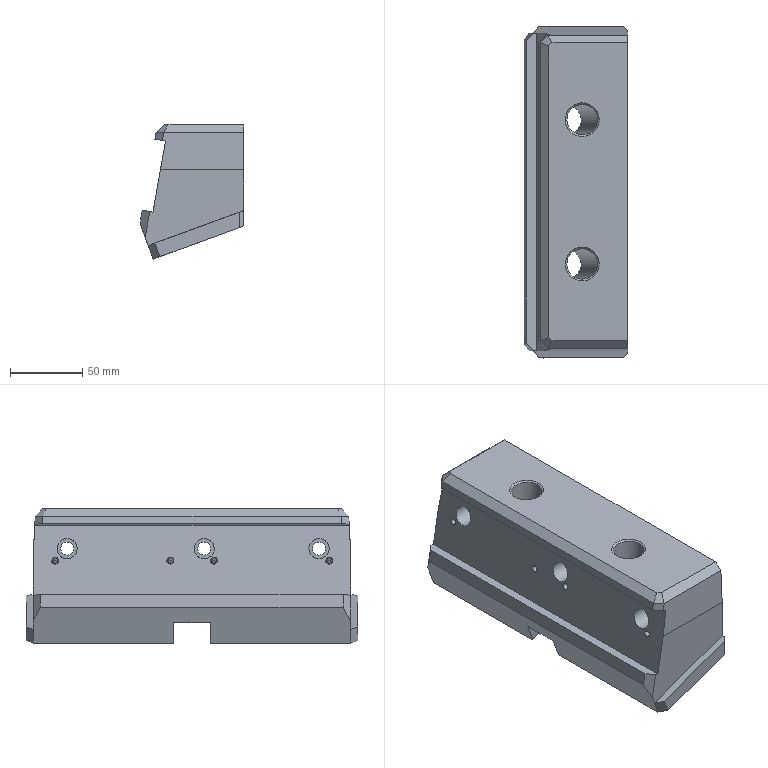Part | STEP file | P011002S003-000 | 1 solid | 218 faces | box 72.003 x 230 x 92.915 mm | volume 964495 mm3 | plane 142 | cylinder 34 | cone 20 | other 20 | spline 2 | commonest cylinder face diameters 6 x12 4.167 x4 4.983 x4 5 x4 9 x3 14 x3